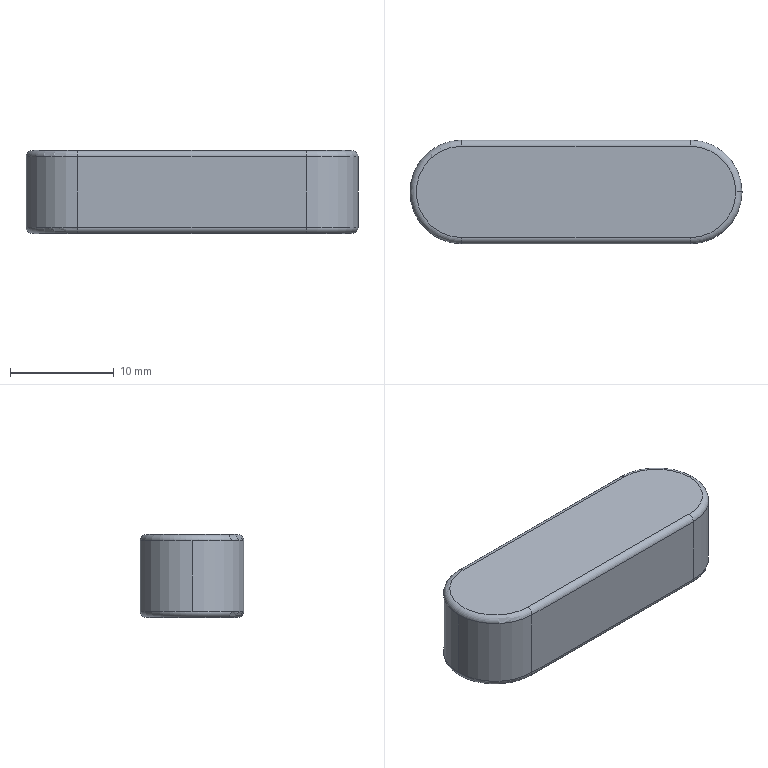Part | SolidWorks | features Extrusion 1, Fillet 1 | 1 solid | 17 faces | box 32 x 10 x 8 mm | volume 2377 mm3 | cylinder 7 | torus 6 | plane 4 | commonest cylinder face diameters 1.2 x4 10 x3
STEP:
#1=CARTESIAN_POINT('',(15.4,0.,0.));
#2=VERTEX_POINT('',#1);
#3=CARTESIAN_POINT('',(11.,-4.4,0.));
#4=VERTEX_POINT('',#3);
#5=CARTESIAN_POINT('',(11.,0.,0.));
#6=DIRECTION('',(0.,0.,-1.));
#7=DIRECTION('',(1.,0.,0.));
#8=AXIS2_PLACEMENT_3D('',#5,#6,#7);
#9=CIRCLE('',#8,4.4);
#10=EDGE_CURVE('',#2,#4,#9,.T.);
#11=ORIENTED_EDGE('',*,*,#10,.F.);
#12=CARTESIAN_POINT('',(16.,0.,0.6));
#13=VERTEX_POINT('',#12);
#14=CARTESIAN_POINT('',(15.4,0.,0.6));
#15=DIRECTION('',(0.,-1.,0.));
#16=DIRECTION('',(0.,0.,-1.));
#17=AXIS2_PLACEMENT_3D('',#14,#15,#16);
#18=CIRCLE('',#17,0.6);
#19=EDGE_CURVE('',#2,#13,#18,.T.);
#20=ORIENTED_EDGE('',*,*,#19,.T.);
#21=CARTESIAN_POINT('',(11.,-5.,0.6));
#22=VERTEX_POINT('',#21);
#23=CARTESIAN_POINT('',(11.,0.,0.6));
#24=DIRECTION('',(0.,0.,1.));
#25=DIRECTION('',(1.,0.,0.));
#26=AXIS2_PLACEMENT_3D('',#23,#24,#25);
#27=CIRCLE('',#26,5.);
#28=EDGE_CURVE('',#22,#13,#27,.T.);
#29=ORIENTED_EDGE('',*,*,#28,.F.);
#30=CARTESIAN_POINT('',(11.,-4.4,0.6));
#31=DIRECTION('',(1.,0.,0.));
#32=DIRECTION('',(0.,0.,-1.));
#33=AXIS2_PLACEMENT_3D('',#30,#31,#32);
#34=CIRCLE('',#33,0.6);
#35=EDGE_CURVE('',#22,#4,#34,.T.);
#36=ORIENTED_EDGE('',*,*,#35,.T.);
#37=EDGE_LOOP('',(#11,#20,#29,#36));
#38=FACE_OUTER_BOUND('',#37,.T.);
#39=CARTESIAN_POINT('',(11.,0.,0.6));
#40=DIRECTION('',(0.,0.,1.));
#41=DIRECTION('',(1.,0.,0.));
#42=AXIS2_PLACEMENT_3D('',#39,#40,#41);
#43=TOROIDAL_SURFACE('',#42,4.4,0.6);
#44=ADVANCED_FACE('',(#38),#43,.T.);
#45=CARTESIAN_POINT('',(16.,0.,7.4));
#46=VERTEX_POINT('',#45);
#47=CARTESIAN_POINT('',(11.,-5.,7.4));
#48=VERTEX_POINT('',#47);
#49=CARTESIAN_POINT('',(11.,0.,7.4));
#50=DIRECTION('',(0.,0.,-1.));
#51=DIRECTION('',(1.,0.,0.));
#52=AXIS2_PLACEMENT_3D('',#49,#50,#51);
#53=CIRCLE('',#52,5.);
#54=EDGE_CURVE('',#46,#48,#53,.T.);
#55=ORIENTED_EDGE('',*,*,#54,.F.);
#56=CARTESIAN_POINT('',(15.4,0.,8.));
#57=VERTEX_POINT('',#56);
#58=CARTESIAN_POINT('',(15.4,0.,7.4));
#59=DIRECTION('',(0.,-1.,0.));
#60=DIRECTION('',(0.,0.,-1.));
#61=AXIS2_PLACEMENT_3D('',#58,#59,#60);
#62=CIRCLE('',#61,0.6);
#63=EDGE_CURVE('',#46,#57,#62,.T.);
#64=ORIENTED_EDGE('',*,*,#63,.T.);
#65=CARTESIAN_POINT('',(11.,-4.4,8.));
#66=VERTEX_POINT('',#65);
#67=CARTESIAN_POINT('',(11.,0.,8.));
#68=DIRECTION('',(0.,0.,1.));
#69=DIRECTION('',(1.,0.,0.));
#70=AXIS2_PLACEMENT_3D('',#67,#68,#69);
#71=CIRCLE('',#70,4.4);
#72=EDGE_CURVE('',#66,#57,#71,.T.);
#73=ORIENTED_EDGE('',*,*,#72,.F.);
#74=CARTESIAN_POINT('',(11.,-4.4,7.4));
#75=DIRECTION('',(1.,0.,0.));
#76=DIRECTION('',(0.,0.,-1.));
#77=AXIS2_PLACEMENT_3D('',#74,#75,#76);
#78=CIRCLE('',#77,0.6);
#79=EDGE_CURVE('',#66,#48,#78,.T.);
#80=ORIENTED_EDGE('',*,*,#79,.T.);
#81=EDGE_LOOP('',(#55,#64,#73,#80));
#82=FACE_OUTER_BOUND('',#81,.T.);
#83=CARTESIAN_POINT('',(11.,0.,7.4));
#84=DIRECTION('',(0.,0.,1.));
#85=DIRECTION('',(1.,0.,0.));
#86=AXIS2_PLACEMENT_3D('',#83,#84,#85);
#87=TOROIDAL_SURFACE('',#86,4.4,0.6);
#88=ADVANCED_FACE('',(#82),#87,.T.);
#89=CARTESIAN_POINT('',(-11.,-5.,7.4));
#90=VERTEX_POINT('',#89);
#91=CARTESIAN_POINT('',(-16.,0.,7.4));
#92=VERTEX_POINT('',#91);
#93=CARTESIAN_POINT('',(-11.,0.,7.4));
#94=DIRECTION('',(0.,0.,-1.));
#95=DIRECTION('',(1.,0.,0.));
#96=AXIS2_PLACEMENT_3D('',#93,#94,#95);
#97=CIRCLE('',#96,5.);
#98=EDGE_CURVE('',#90,#92,#97,.T.);
#99=ORIENTED_EDGE('',*,*,#98,.T.);
#100=CARTESIAN_POINT('',(-16.,0.,0.6));
#101=VERTEX_POINT('',#100);
#102=CARTESIAN_POINT('',(-16.,0.,8.));
#103=DIRECTION('',(0.,0.,-1.));
#104=VECTOR('',#103,1000.);
#105=LINE('',#102,#104);
#106=EDGE_CURVE('',#92,#101,#105,.T.);
#107=ORIENTED_EDGE('',*,*,#106,.T.);
#108=CARTESIAN_POINT('',(-11.,-5.,0.6));
#109=VERTEX_POINT('',#108);
#110=CARTESIAN_POINT('',(-11.,0.,0.6));
#111=DIRECTION('',(0.,0.,1.));
#112=DIRECTION('',(1.,0.,0.));
#113=AXIS2_PLACEMENT_3D('',#110,#111,#112);
#114=CIRCLE('',#113,5.);
#115=EDGE_CURVE('',#101,#109,#114,.T.);
#116=ORIENTED_EDGE('',*,*,#115,.T.);
#117=CARTESIAN_POINT('',(-11.,-5.,8.));
#118=DIRECTION('',(0.,0.,-1.));
#119=VECTOR('',#118,1000.);
#120=LINE('',#117,#119);
#121=EDGE_CURVE('',#90,#109,#120,.T.);
#122=ORIENTED_EDGE('',*,*,#121,.F.);
#123=EDGE_LOOP('',(#99,#107,#116,#122));
#124=FACE_OUTER_BOUND('',#123,.T.);
#125=CARTESIAN_POINT('',(-11.,0.,8.));
#126=DIRECTION('',(0.,0.,-1.));
#127=DIRECTION('',(-1.,0.,0.));
#128=AXIS2_PLACEMENT_3D('',#125,#126,#127);
#129=CYLINDRICAL_SURFACE('',#128,5.);
#130=ADVANCED_FACE('',(#124),#129,.T.);
#131=ORIENTED_EDGE('',*,*,#106,.F.);
#132=CARTESIAN_POINT('',(-11.,5.,7.4));
#133=VERTEX_POINT('',#132);
#134=CARTESIAN_POINT('',(-11.,0.,7.4));
#135=DIRECTION('',(0.,0.,-1.));
#136=DIRECTION('',(1.,0.,0.));
#137=AXIS2_PLACEMENT_3D('',#134,#135,#136);
#138=CIRCLE('',#137,5.);
#139=EDGE_CURVE('',#92,#133,#138,.T.);
#140=ORIENTED_EDGE('',*,*,#139,.T.);
#141=CARTESIAN_POINT('',(-11.,5.,0.6));
#142=VERTEX_POINT('',#141);
#143=CARTESIAN_POINT('',(-11.,5.,8.));
#144=DIRECTION('',(0.,0.,-1.));
#145=VECTOR('',#144,1000.);
#146=LINE('',#143,#145);
#147=EDGE_CURVE('',#133,#142,#146,.T.);
#148=ORIENTED_EDGE('',*,*,#147,.T.);
#149=CARTESIAN_POINT('',(-11.,0.,0.6));
#150=DIRECTION('',(0.,0.,1.));
#151=DIRECTION('',(1.,0.,0.));
#152=AXIS2_PLACEMENT_3D('',#149,#150,#151);
#153=CIRCLE('',#152,5.);
#154=EDGE_CURVE('',#142,#101,#153,.T.);
#155=ORIENTED_EDGE('',*,*,#154,.T.);
#156=EDGE_LOOP('',(#131,#140,#148,#155));
#157=FACE_OUTER_BOUND('',#156,.T.);
#158=CARTESIAN_POINT('',(-11.,0.,8.));
#159=DIRECTION('',(0.,0.,-1.));
#160=DIRECTION('',(-1.,0.,0.));
#161=AXIS2_PLACEMENT_3D('',#158,#159,#160);
#162=CYLINDRICAL_SURFACE('',#161,5.);
#163=ADVANCED_FACE('',(#157),#162,.T.);
#164=CARTESIAN_POINT('',(11.,-5.,8.));
#165=DIRECTION('',(0.,0.,-1.));
#166=VECTOR('',#165,1000.);
#167=LINE('',#164,#166);
#168=EDGE_CURVE('',#48,#22,#167,.T.);
#169=ORIENTED_EDGE('',*,*,#168,.F.);
#170=CARTESIAN_POINT('',(-11.,-5.,7.4));
#171=DIRECTION('',(-1.,0.,0.));
#172=VECTOR('',#171,1000.);
#173=LINE('',#170,#172);
#174=EDGE_CURVE('',#48,#90,#173,.T.);
#175=ORIENTED_EDGE('',*,*,#174,.T.);
#176=ORIENTED_EDGE('',*,*,#121,.T.);
#177=CARTESIAN_POINT('',(-11.,-5.,0.6));
#178=DIRECTION('',(1.,0.,0.));
#179=VECTOR('',#178,1000.);
#180=LINE('',#177,#179);
#181=EDGE_CURVE('',#109,#22,#180,.T.);
#182=ORIENTED_EDGE('',*,*,#181,.T.);
#183=EDGE_LOOP('',(#169,#175,#176,#182));
#184=FACE_OUTER_BOUND('',#183,.T.);
#185=CARTESIAN_POINT('',(-11.,-5.,8.));
#186=DIRECTION('',(0.,1.,0.));
#187=DIRECTION('',(-1.,0.,0.));
#188=AXIS2_PLACEMENT_3D('',#185,#186,#187);
#189=PLANE('',#188);
#190=ADVANCED_FACE('',(#184),#189,.F.);
#191=CARTESIAN_POINT('',(11.,5.,7.4));
#192=VERTEX_POINT('',#191);
#193=CARTESIAN_POINT('',(11.,5.,0.6));
#194=VERTEX_POINT('',#193);
#195=CARTESIAN_POINT('',(11.,5.,8.));
#196=DIRECTION('',(0.,0.,-1.));
#197=VECTOR('',#196,1000.);
#198=LINE('',#195,#197);
#199=EDGE_CURVE('',#192,#194,#198,.T.);
#200=ORIENTED_EDGE('',*,*,#199,.F.);
#201=CARTESIAN_POINT('',(11.,0.,7.4));
#202=DIRECTION('',(0.,0.,-1.));
#203=DIRECTION('',(1.,0.,0.));
#204=AXIS2_PLACEMENT_3D('',#201,#202,#203);
#205=CIRCLE('',#204,5.);
#206=EDGE_CURVE('',#192,#46,#205,.T.);
#207=ORIENTED_EDGE('',*,*,#206,.T.);
#208=ORIENTED_EDGE('',*,*,#54,.T.);
#209=ORIENTED_EDGE('',*,*,#168,.T.);
#210=ORIENTED_EDGE('',*,*,#28,.T.);
#211=CARTESIAN_POINT('',(11.,0.,0.6));
#212=DIRECTION('',(0.,0.,1.));
#213=DIRECTION('',(1.,0.,0.));
#214=AXIS2_PLACEMENT_3D('',#211,#212,#213);
#215=CIRCLE('',#214,5.);
#216=EDGE_CURVE('',#13,#194,#215,.T.);
#217=ORIENTED_EDGE('',*,*,#216,.T.);
#218=EDGE_LOOP('',(#200,#207,#208,#209,#210,#217));
#219=FACE_OUTER_BOUND('',#218,.T.);
#220=CARTESIAN_POINT('',(11.,0.,8.));
#221=DIRECTION('',(0.,0.,-1.));
#222=DIRECTION('',(-1.,0.,0.));
#223=AXIS2_PLACEMENT_3D('',#220,#221,#222);
#224=CYLINDRICAL_SURFACE('',#223,5.);
#225=ADVANCED_FACE('',(#219),#224,.T.);
#226=ORIENTED_EDGE('',*,*,#147,.F.);
#227=CARTESIAN_POINT('',(11.,5.,7.4));
#228=DIRECTION('',(1.,0.,0.));
#229=VECTOR('',#228,1000.);
#230=LINE('',#227,#229);
#231=EDGE_CURVE('',#133,#192,#230,.T.);
#232=ORIENTED_EDGE('',*,*,#231,.T.);
#233=ORIENTED_EDGE('',*,*,#199,.T.);
#234=CARTESIAN_POINT('',(-11.,5.,0.6));
#235=DIRECTION('',(-1.,0.,0.));
#236=VECTOR('',#235,1000.);
#237=LINE('',#234,#236);
#238=EDGE_CURVE('',#194,#142,#237,.T.);
#239=ORIENTED_EDGE('',*,*,#238,.T.);
#240=EDGE_LOOP('',(#226,#232,#233,#239));
#241=FACE_OUTER_BOUND('',#240,.T.);
#242=CARTESIAN_POINT('',(-11.,5.,8.));
#243=DIRECTION('',(0.,-1.,0.));
#244=DIRECTION('',(1.,0.,0.));
#245=AXIS2_PLACEMENT_3D('',#242,#243,#244);
#246=PLANE('',#245);
#247=ADVANCED_FACE('',(#241),#246,.F.);
#248=CARTESIAN_POINT('',(-11.,-4.4,8.));
#249=VERTEX_POINT('',#248);
#250=CARTESIAN_POINT('',(11.,-4.4,8.));
#251=DIRECTION('',(1.,0.,0.));
#252=VECTOR('',#251,1000.);
#253=LINE('',#250,#252);
#254=EDGE_CURVE('',#249,#66,#253,.T.);
#255=ORIENTED_EDGE('',*,*,#254,.T.);
#256=ORIENTED_EDGE('',*,*,#72,.T.);
#257=CARTESIAN_POINT('',(11.,4.4,8.));
#258=VERTEX_POINT('',#257);
#259=CARTESIAN_POINT('',(11.,0.,8.));
#260=DIRECTION('',(0.,0.,1.));
#261=DIRECTION('',(1.,0.,0.));
#262=AXIS2_PLACEMENT_3D('',#259,#260,#261);
#263=CIRCLE('',#262,4.4);
#264=EDGE_CURVE('',#57,#258,#263,.T.);
#265=ORIENTED_EDGE('',*,*,#264,.T.);
#266=CARTESIAN_POINT('',(-11.,4.4,8.));
#267=VERTEX_POINT('',#266);
#268=CARTESIAN_POINT('',(-11.,4.4,8.));
#269=DIRECTION('',(-1.,0.,0.));
#270=VECTOR('',#269,1000.);
#271=LINE('',#268,#270);
#272=EDGE_CURVE('',#258,#267,#271,.T.);
#273=ORIENTED_EDGE('',*,*,#272,.T.);
#274=CARTESIAN_POINT('',(-11.,0.,8.));
#275=DIRECTION('',(0.,0.,1.));
#276=DIRECTION('',(1.,0.,0.));
#277=AXIS2_PLACEMENT_3D('',#274,#275,#276);
#278=CIRCLE('',#277,4.4);
#279=EDGE_CURVE('',#267,#249,#278,.T.);
#280=ORIENTED_EDGE('',*,*,#279,.T.);
#281=EDGE_LOOP('',(#255,#256,#265,#273,#280));
#282=FACE_OUTER_BOUND('',#281,.T.);
#283=CARTESIAN_POINT('',(-11.,0.,8.));
#284=DIRECTION('',(0.,0.,1.));
#285=DIRECTION('',(1.,0.,0.));
#286=AXIS2_PLACEMENT_3D('',#283,#284,#285);
#287=PLANE('',#286);
#288=ADVANCED_FACE('',(#282),#287,.T.);
#289=CARTESIAN_POINT('',(-11.,4.4,0.));
#290=VERTEX_POINT('',#289);
#291=CARTESIAN_POINT('',(11.,4.4,0.));
#292=VERTEX_POINT('',#291);
#293=CARTESIAN_POINT('',(-11.,4.4,0.));
#294=DIRECTION('',(1.,0.,0.));
#295=VECTOR('',#294,1000.);
#296=LINE('',#293,#295);
#297=EDGE_CURVE('',#290,#292,#296,.T.);
#298=ORIENTED_EDGE('',*,*,#297,.T.);
#299=CARTESIAN_POINT('',(11.,0.,0.));
#300=DIRECTION('',(0.,0.,-1.));
#301=DIRECTION('',(1.,0.,0.));
#302=AXIS2_PLACEMENT_3D('',#299,#300,#301);
#303=CIRCLE('',#302,4.4);
#304=EDGE_CURVE('',#292,#2,#303,.T.);
#305=ORIENTED_EDGE('',*,*,#304,.T.);
#306=ORIENTED_EDGE('',*,*,#10,.T.);
#307=CARTESIAN_POINT('',(-11.,-4.4,0.));
#308=VERTEX_POINT('',#307);
#309=CARTESIAN_POINT('',(-11.,-4.4,0.));
#310=DIRECTION('',(-1.,0.,0.));
#311=VECTOR('',#310,1000.);
#312=LINE('',#309,#311);
#313=EDGE_CURVE('',#4,#308,#312,.T.);
#314=ORIENTED_EDGE('',*,*,#313,.T.);
#315=CARTESIAN_POINT('',(-11.,0.,0.));
#316=DIRECTION('',(0.,0.,-1.));
#317=DIRECTION('',(1.,0.,0.));
#318=AXIS2_PLACEMENT_3D('',#315,#316,#317);
#319=CIRCLE('',#318,4.4);
#320=EDGE_CURVE('',#308,#290,#319,.T.);
#321=ORIENTED_EDGE('',*,*,#320,.T.);
#322=EDGE_LOOP('',(#298,#305,#306,#314,#321));
#323=FACE_OUTER_BOUND('',#322,.T.);
#324=CARTESIAN_POINT('',(-11.,0.,0.));
#325=DIRECTION('',(0.,0.,1.));
#326=DIRECTION('',(1.,0.,0.));
#327=AXIS2_PLACEMENT_3D('',#324,#325,#326);
#328=PLANE('',#327);
#329=ADVANCED_FACE('',(#323),#328,.F.);
#330=CARTESIAN_POINT('',(-11.,4.4,7.4));
#331=DIRECTION('',(1.,0.,0.));
#332=DIRECTION('',(0.,0.,-1.));
#333=AXIS2_PLACEMENT_3D('',#330,#331,#332);
#334=CIRCLE('',#333,0.6);
#335=EDGE_CURVE('',#133,#267,#334,.T.);
#336=ORIENTED_EDGE('',*,*,#335,.F.);
#337=ORIENTED_EDGE('',*,*,#139,.F.);
#338=ORIENTED_EDGE('',*,*,#98,.F.);
#339=CARTESIAN_POINT('',(-11.,-4.4,7.4));
#340=DIRECTION('',(1.,0.,0.));
#341=DIRECTION('',(0.,0.,-1.));
#342=AXIS2_PLACEMENT_3D('',#339,#340,#341);
#343=CIRCLE('',#342,0.6);
#344=EDGE_CURVE('',#249,#90,#343,.T.);
#345=ORIENTED_EDGE('',*,*,#344,.F.);
#346=ORIENTED_EDGE('',*,*,#279,.F.);
#347=EDGE_LOOP('',(#336,#337,#338,#345,#346));
#348=FACE_OUTER_BOUND('',#347,.T.);
#349=CARTESIAN_POINT('',(-11.,0.,7.4));
#350=DIRECTION('',(0.,0.,1.));
#351=DIRECTION('',(1.,0.,0.));
#352=AXIS2_PLACEMENT_3D('',#349,#350,#351);
#353=TOROIDAL_SURFACE('',#352,4.4,0.6);
#354=ADVANCED_FACE('',(#348),#353,.T.);
#355=ORIENTED_EDGE('',*,*,#344,.T.);
#356=ORIENTED_EDGE('',*,*,#174,.F.);
#357=ORIENTED_EDGE('',*,*,#79,.F.);
#358=ORIENTED_EDGE('',*,*,#254,.F.);
#359=EDGE_LOOP('',(#355,#356,#357,#358));
#360=FACE_OUTER_BOUND('',#359,.T.);
#361=CARTESIAN_POINT('',(-11.,-4.4,7.4));
#362=DIRECTION('',(-1.,0.,0.));
#363=DIRECTION('',(0.,-1.,0.));
#364=AXIS2_PLACEMENT_3D('',#361,#362,#363);
#365=CYLINDRICAL_SURFACE('',#364,0.6);
#366=ADVANCED_FACE('',(#360),#365,.T.);
#367=ORIENTED_EDGE('',*,*,#335,.T.);
#368=ORIENTED_EDGE('',*,*,#272,.F.);
#369=CARTESIAN_POINT('',(11.,4.4,7.4));
#370=DIRECTION('',(1.,0.,0.));
#371=DIRECTION('',(0.,0.,-1.));
#372=AXIS2_PLACEMENT_3D('',#369,#370,#371);
#373=CIRCLE('',#372,0.6);
#374=EDGE_CURVE('',#192,#258,#373,.T.);
#375=ORIENTED_EDGE('',*,*,#374,.F.);
#376=ORIENTED_EDGE('',*,*,#231,.F.);
#377=EDGE_LOOP('',(#367,#368,#375,#376));
#378=FACE_OUTER_BOUND('',#377,.T.);
#379=CARTESIAN_POINT('',(-11.,4.4,7.4));
#380=DIRECTION('',(1.,0.,0.));
#381=DIRECTION('',(0.,1.,0.));
#382=AXIS2_PLACEMENT_3D('',#379,#380,#381);
#383=CYLINDRICAL_SURFACE('',#382,0.6);
#384=ADVANCED_FACE('',(#378),#383,.T.);
#385=ORIENTED_EDGE('',*,*,#63,.F.);
#386=ORIENTED_EDGE('',*,*,#206,.F.);
#387=ORIENTED_EDGE('',*,*,#374,.T.);
#388=ORIENTED_EDGE('',*,*,#264,.F.);
#389=EDGE_LOOP('',(#385,#386,#387,#388));
#390=FACE_OUTER_BOUND('',#389,.T.);
#391=CARTESIAN_POINT('',(11.,0.,7.4));
#392=DIRECTION('',(0.,0.,1.));
#393=DIRECTION('',(1.,0.,0.));
#394=AXIS2_PLACEMENT_3D('',#391,#392,#393);
#395=TOROIDAL_SURFACE('',#394,4.4,0.6);
#396=ADVANCED_FACE('',(#390),#395,.T.);
#397=CARTESIAN_POINT('',(-11.,4.4,0.6));
#398=DIRECTION('',(1.,0.,0.));
#399=DIRECTION('',(0.,0.,-1.));
#400=AXIS2_PLACEMENT_3D('',#397,#398,#399);
#401=CIRCLE('',#400,0.6);
#402=EDGE_CURVE('',#290,#142,#401,.T.);
#403=ORIENTED_EDGE('',*,*,#402,.F.);
#404=ORIENTED_EDGE('',*,*,#320,.F.);
#405=CARTESIAN_POINT('',(-11.,-4.4,0.6));
#406=DIRECTION('',(1.,0.,0.));
#407=DIRECTION('',(0.,0.,-1.));
#408=AXIS2_PLACEMENT_3D('',#405,#406,#407);
#409=CIRCLE('',#408,0.6);
#410=EDGE_CURVE('',#109,#308,#409,.T.);
#411=ORIENTED_EDGE('',*,*,#410,.F.);
#412=ORIENTED_EDGE('',*,*,#115,.F.);
#413=ORIENTED_EDGE('',*,*,#154,.F.);
#414=EDGE_LOOP('',(#403,#404,#411,#412,#413));
#415=FACE_OUTER_BOUND('',#414,.T.);
#416=CARTESIAN_POINT('',(-11.,0.,0.6));
#417=DIRECTION('',(0.,0.,1.));
#418=DIRECTION('',(1.,0.,0.));
#419=AXIS2_PLACEMENT_3D('',#416,#417,#418);
#420=TOROIDAL_SURFACE('',#419,4.4,0.6);
#421=ADVANCED_FACE('',(#415),#420,.T.);
#422=ORIENTED_EDGE('',*,*,#410,.T.);
#423=ORIENTED_EDGE('',*,*,#313,.F.);
#424=ORIENTED_EDGE('',*,*,#35,.F.);
#425=ORIENTED_EDGE('',*,*,#181,.F.);
#426=EDGE_LOOP('',(#422,#423,#424,#425));
#427=FACE_OUTER_BOUND('',#426,.T.);
#428=CARTESIAN_POINT('',(-11.,-4.4,0.6));
#429=DIRECTION('',(1.,0.,0.));
#430=DIRECTION('',(0.,1.,0.));
#431=AXIS2_PLACEMENT_3D('',#428,#429,#430);
#432=CYLINDRICAL_SURFACE('',#431,0.6);
#433=ADVANCED_FACE('',(#427),#432,.T.);
#434=ORIENTED_EDGE('',*,*,#402,.T.);
#435=ORIENTED_EDGE('',*,*,#238,.F.);
#436=CARTESIAN_POINT('',(11.,4.4,0.6));
#437=DIRECTION('',(1.,0.,0.));
#438=DIRECTION('',(0.,0.,-1.));
#439=AXIS2_PLACEMENT_3D('',#436,#437,#438);
#440=CIRCLE('',#439,0.6);
#441=EDGE_CURVE('',#292,#194,#440,.T.);
#442=ORIENTED_EDGE('',*,*,#441,.F.);
#443=ORIENTED_EDGE('',*,*,#297,.F.);
#444=EDGE_LOOP('',(#434,#435,#442,#443));
#445=FACE_OUTER_BOUND('',#444,.T.);
#446=CARTESIAN_POINT('',(-11.,4.4,0.6));
#447=DIRECTION('',(-1.,0.,0.));
#448=DIRECTION('',(0.,-1.,0.));
#449=AXIS2_PLACEMENT_3D('',#446,#447,#448);
#450=CYLINDRICAL_SURFACE('',#449,0.6);
#451=ADVANCED_FACE('',(#445),#450,.T.);
#452=ORIENTED_EDGE('',*,*,#19,.F.);
#453=ORIENTED_EDGE('',*,*,#304,.F.);
#454=ORIENTED_EDGE('',*,*,#441,.T.);
#455=ORIENTED_EDGE('',*,*,#216,.F.);
#456=EDGE_LOOP('',(#452,#453,#454,#455));
#457=FACE_OUTER_BOUND('',#456,.T.);
#458=CARTESIAN_POINT('',(11.,0.,0.6));
#459=DIRECTION('',(0.,0.,1.));
#460=DIRECTION('',(1.,0.,0.));
#461=AXIS2_PLACEMENT_3D('',#458,#459,#460);
#462=TOROIDAL_SURFACE('',#461,4.4,0.6);
#463=ADVANCED_FACE('',(#457),#462,.T.);
#464=CLOSED_SHELL('',(#44,#88,#130,#163,#190,#225,#247,#288,#329,#354,#366,#384,#396,#421,#433,#451,#463));
#465=MANIFOLD_SOLID_BREP('',#464);
#466=CARTESIAN_POINT('',(0.,0.,0.));
#467=DIRECTION('',(0.,0.,1.));
#468=DIRECTION('',(1.,0.,0.));
#469=AXIS2_PLACEMENT_3D('',#466,#467,#468);
#470=(LENGTH_UNIT()NAMED_UNIT(*)SI_UNIT(.MILLI.,.METRE.));
#471=UNCERTAINTY_MEASURE_WITH_UNIT(LENGTH_MEASURE(0.00001),#470,'','');
#472=(NAMED_UNIT(*)PLANE_ANGLE_UNIT()SI_UNIT($,.RADIAN.));
#473=(NAMED_UNIT(*)SI_UNIT($,.STERADIAN.)SOLID_ANGLE_UNIT());
#474=(GEOMETRIC_REPRESENTATION_CONTEXT(3)GLOBAL_UNCERTAINTY_ASSIGNED_CONTEXT((#471))GLOBAL_UNIT_ASSIGNED_CONTEXT((#470,#472,#473))REPRESENTATION_CONTEXT('',''));
#475=ADVANCED_BREP_SHAPE_REPRESENTATION('',(#465,#469),#474);